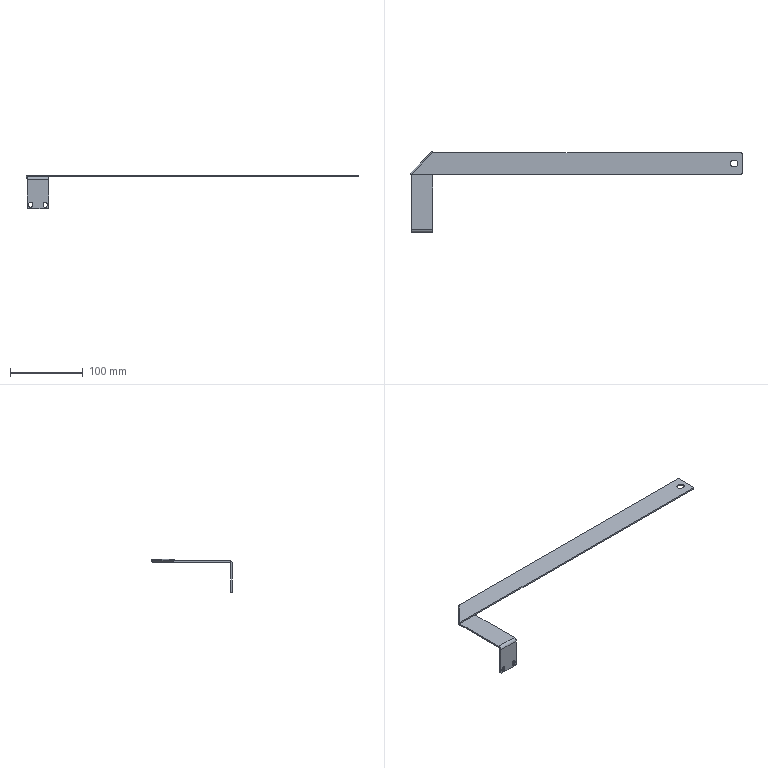Part | NX | features BREP 1 | 1 solid | 37 faces | box 457.646 x 111.304 x 46.082 mm | volume 34595 mm3 | plane 20 | cylinder 17 | commonest cylinder face diameters 5.5 x6 4 x5 9 x3 2 x2 8 x1
STEP:
#1=CARTESIAN_POINT('',(-257.062,-128.404,2032.018));
#2=VERTEX_POINT('',#1);
#3=CARTESIAN_POINT('',(-258.476,-126.99,2034.018));
#4=VERTEX_POINT('',#3);
#5=CARTESIAN_POINT('',(-257.062,-128.404,2034.018));
#6=DIRECTION('',(0.7071,0.7071,0.));
#7=DIRECTION('',(-0.7071,0.7071,0.));
#8=AXIS2_PLACEMENT_3D('',#5,#6,#7);
#9=CIRCLE('',#8,2.);
#10=EDGE_CURVE('',#2,#4,#9,.T.);
#11=ORIENTED_EDGE('',*,*,#10,.T.);
#12=CARTESIAN_POINT('',(-228.476,-96.99,2034.018));
#13=VERTEX_POINT('',#12);
#14=CARTESIAN_POINT('',(-258.476,-126.99,2034.018));
#15=DIRECTION('',(0.7071,0.7071,0.));
#16=VECTOR('',#15,1000.);
#17=LINE('',#14,#16);
#18=EDGE_CURVE('',#4,#13,#17,.T.);
#19=ORIENTED_EDGE('',*,*,#18,.T.);
#20=CARTESIAN_POINT('',(-227.062,-98.404,2032.018));
#21=VERTEX_POINT('',#20);
#22=CARTESIAN_POINT('',(-227.062,-98.404,2034.018));
#23=DIRECTION('',(-0.7071,-0.7071,0.));
#24=DIRECTION('',(-0.7071,0.7071,0.));
#25=AXIS2_PLACEMENT_3D('',#22,#23,#24);
#26=CIRCLE('',#25,2.);
#27=EDGE_CURVE('',#13,#21,#26,.T.);
#28=ORIENTED_EDGE('',*,*,#27,.T.);
#29=CARTESIAN_POINT('',(-257.062,-128.404,2032.018));
#30=DIRECTION('',(-0.7071,-0.7071,0.));
#31=VECTOR('',#30,1000.);
#32=LINE('',#29,#31);
#33=EDGE_CURVE('',#21,#2,#32,.T.);
#34=ORIENTED_EDGE('',*,*,#33,.T.);
#35=EDGE_LOOP('',(#11,#19,#28,#34));
#36=FACE_BOUND('',#35,.T.);
#37=CARTESIAN_POINT('',(-257.062,-128.404,2034.018));
#38=DIRECTION('',(0.7071,0.7071,0.));
#39=DIRECTION('',(0.7071,-0.7071,0.));
#40=AXIS2_PLACEMENT_3D('',#37,#38,#39);
#41=CYLINDRICAL_SURFACE('',#40,2.);
#42=ADVANCED_FACE('',(#36),#41,.T.);
#43=CARTESIAN_POINT('',(193.42,-113.404,2034.018));
#44=VERTEX_POINT('',#43);
#45=CARTESIAN_POINT('',(188.92,-108.904,2034.018));
#46=VERTEX_POINT('',#45);
#47=CARTESIAN_POINT('',(188.92,-113.404,2034.018));
#48=DIRECTION('',(0.,0.,1.));
#49=DIRECTION('',(1.,0.,0.));
#50=AXIS2_PLACEMENT_3D('',#47,#48,#49);
#51=CIRCLE('',#50,4.5);
#52=EDGE_CURVE('',#44,#46,#51,.T.);
#53=ORIENTED_EDGE('',*,*,#52,.F.);
#54=CARTESIAN_POINT('',(193.42,-113.404,2036.018));
#55=VERTEX_POINT('',#54);
#56=CARTESIAN_POINT('',(193.42,-113.404,2035.018));
#57=DIRECTION('',(0.,0.,1.));
#58=VECTOR('',#57,1000.);
#59=LINE('',#56,#58);
#60=EDGE_CURVE('',#44,#55,#59,.T.);
#61=ORIENTED_EDGE('',*,*,#60,.T.);
#62=CARTESIAN_POINT('',(188.92,-108.904,2036.018));
#63=VERTEX_POINT('',#62);
#64=CARTESIAN_POINT('',(188.92,-113.404,2036.018));
#65=DIRECTION('',(0.,0.,1.));
#66=DIRECTION('',(1.,0.,0.));
#67=AXIS2_PLACEMENT_3D('',#64,#65,#66);
#68=CIRCLE('',#67,4.5);
#69=EDGE_CURVE('',#55,#63,#68,.T.);
#70=ORIENTED_EDGE('',*,*,#69,.T.);
#71=CARTESIAN_POINT('',(188.92,-108.904,2035.018));
#72=DIRECTION('',(0.,0.,1.));
#73=VECTOR('',#72,1000.);
#74=LINE('',#71,#73);
#75=EDGE_CURVE('',#46,#63,#74,.T.);
#76=ORIENTED_EDGE('',*,*,#75,.F.);
#77=EDGE_LOOP('',(#53,#61,#70,#76));
#78=FACE_BOUND('',#77,.T.);
#79=CARTESIAN_POINT('',(188.92,-113.404,2035.018));
#80=DIRECTION('',(0.,0.,1.));
#81=DIRECTION('',(-1.,0.,0.));
#82=AXIS2_PLACEMENT_3D('',#79,#80,#81);
#83=CYLINDRICAL_SURFACE('',#82,4.5);
#84=ADVANCED_FACE('',(#78),#83,.F.);
#85=CARTESIAN_POINT('',(-229.312,-206.294,1994.768));
#86=VERTEX_POINT('',#85);
#87=CARTESIAN_POINT('',(-232.062,-206.294,1992.018));
#88=VERTEX_POINT('',#87);
#89=CARTESIAN_POINT('',(-232.062,-206.294,1994.768));
#90=DIRECTION('',(0.,1.,0.));
#91=DIRECTION('',(0.,0.,-1.));
#92=AXIS2_PLACEMENT_3D('',#89,#90,#91);
#93=CIRCLE('',#92,2.75);
#94=EDGE_CURVE('',#86,#88,#93,.T.);
#95=ORIENTED_EDGE('',*,*,#94,.T.);
#96=CARTESIAN_POINT('',(-232.062,-208.294,1992.018));
#97=VERTEX_POINT('',#96);
#98=CARTESIAN_POINT('',(-232.062,-207.294,1992.018));
#99=DIRECTION('',(0.,-1.,0.));
#100=VECTOR('',#99,1000.);
#101=LINE('',#98,#100);
#102=EDGE_CURVE('',#88,#97,#101,.T.);
#103=ORIENTED_EDGE('',*,*,#102,.T.);
#104=CARTESIAN_POINT('',(-229.312,-208.294,1994.768));
#105=VERTEX_POINT('',#104);
#106=CARTESIAN_POINT('',(-232.062,-208.294,1994.768));
#107=DIRECTION('',(0.,1.,0.));
#108=DIRECTION('',(0.,0.,-1.));
#109=AXIS2_PLACEMENT_3D('',#106,#107,#108);
#110=CIRCLE('',#109,2.75);
#111=EDGE_CURVE('',#105,#97,#110,.T.);
#112=ORIENTED_EDGE('',*,*,#111,.F.);
#113=CARTESIAN_POINT('',(-229.312,-207.294,1994.768));
#114=DIRECTION('',(0.,-1.,0.));
#115=VECTOR('',#114,1000.);
#116=LINE('',#113,#115);
#117=EDGE_CURVE('',#86,#105,#116,.T.);
#118=ORIENTED_EDGE('',*,*,#117,.F.);
#119=EDGE_LOOP('',(#95,#103,#112,#118));
#120=FACE_BOUND('',#119,.T.);
#121=CARTESIAN_POINT('',(-232.062,-207.294,1994.768));
#122=DIRECTION('',(0.,-1.,0.));
#123=DIRECTION('',(0.,0.,1.));
#124=AXIS2_PLACEMENT_3D('',#121,#122,#123);
#125=CYLINDRICAL_SURFACE('',#124,2.75);
#126=ADVANCED_FACE('',(#120),#125,.F.);
#127=CARTESIAN_POINT('',(-249.312,-206.294,1994.768));
#128=VERTEX_POINT('',#127);
#129=CARTESIAN_POINT('',(-252.062,-206.294,1992.018));
#130=VERTEX_POINT('',#129);
#131=CARTESIAN_POINT('',(-252.062,-206.294,1994.768));
#132=DIRECTION('',(0.,1.,0.));
#133=DIRECTION('',(0.,0.,-1.));
#134=AXIS2_PLACEMENT_3D('',#131,#132,#133);
#135=CIRCLE('',#134,2.75);
#136=EDGE_CURVE('',#128,#130,#135,.T.);
#137=ORIENTED_EDGE('',*,*,#136,.T.);
#138=CARTESIAN_POINT('',(-252.062,-208.294,1992.018));
#139=VERTEX_POINT('',#138);
#140=CARTESIAN_POINT('',(-252.062,-207.294,1992.018));
#141=DIRECTION('',(0.,-1.,0.));
#142=VECTOR('',#141,1000.);
#143=LINE('',#140,#142);
#144=EDGE_CURVE('',#130,#139,#143,.T.);
#145=ORIENTED_EDGE('',*,*,#144,.T.);
#146=CARTESIAN_POINT('',(-249.312,-208.294,1994.768));
#147=VERTEX_POINT('',#146);
#148=CARTESIAN_POINT('',(-252.062,-208.294,1994.768));
#149=DIRECTION('',(0.,1.,0.));
#150=DIRECTION('',(0.,0.,-1.));
#151=AXIS2_PLACEMENT_3D('',#148,#149,#150);
#152=CIRCLE('',#151,2.75);
#153=EDGE_CURVE('',#147,#139,#152,.T.);
#154=ORIENTED_EDGE('',*,*,#153,.F.);
#155=CARTESIAN_POINT('',(-249.312,-207.294,1994.768));
#156=DIRECTION('',(0.,-1.,0.));
#157=VECTOR('',#156,1000.);
#158=LINE('',#155,#157);
#159=EDGE_CURVE('',#128,#147,#158,.T.);
#160=ORIENTED_EDGE('',*,*,#159,.F.);
#161=EDGE_LOOP('',(#137,#145,#154,#160));
#162=FACE_BOUND('',#161,.T.);
#163=CARTESIAN_POINT('',(-252.062,-207.294,1994.768));
#164=DIRECTION('',(0.,-1.,0.));
#165=DIRECTION('',(0.,0.,1.));
#166=AXIS2_PLACEMENT_3D('',#163,#164,#165);
#167=CYLINDRICAL_SURFACE('',#166,2.75);
#168=ADVANCED_FACE('',(#162),#167,.F.);
#169=CARTESIAN_POINT('',(198.17,-128.404,2036.018));
#170=VERTEX_POINT('',#169);
#171=CARTESIAN_POINT('',(-257.062,-128.404,2036.018));
#172=VERTEX_POINT('',#171);
#173=CARTESIAN_POINT('',(-234.19,-128.404,2036.018));
#174=DIRECTION('',(-1.,0.,0.));
#175=VECTOR('',#174,1000.);
#176=LINE('',#173,#175);
#177=EDGE_CURVE('',#170,#172,#176,.T.);
#178=ORIENTED_EDGE('',*,*,#177,.F.);
#179=CARTESIAN_POINT('',(199.17,-127.404,2036.018));
#180=VERTEX_POINT('',#179);
#181=CARTESIAN_POINT('',(198.17,-127.404,2036.018));
#182=DIRECTION('',(0.,0.,-1.));
#183=DIRECTION('',(1.,0.,0.));
#184=AXIS2_PLACEMENT_3D('',#181,#182,#183);
#185=CIRCLE('',#184,1.);
#186=EDGE_CURVE('',#180,#170,#185,.T.);
#187=ORIENTED_EDGE('',*,*,#186,.F.);
#188=CARTESIAN_POINT('',(199.17,-99.404,2036.018));
#189=VERTEX_POINT('',#188);
#190=CARTESIAN_POINT('',(199.17,-105.532,2036.018));
#191=DIRECTION('',(0.,-1.,0.));
#192=VECTOR('',#191,1000.);
#193=LINE('',#190,#192);
#194=EDGE_CURVE('',#189,#180,#193,.T.);
#195=ORIENTED_EDGE('',*,*,#194,.F.);
#196=CARTESIAN_POINT('',(198.17,-98.404,2036.018));
#197=VERTEX_POINT('',#196);
#198=CARTESIAN_POINT('',(198.17,-99.404,2036.018));
#199=DIRECTION('',(0.,0.,-1.));
#200=DIRECTION('',(1.,0.,0.));
#201=AXIS2_PLACEMENT_3D('',#198,#199,#200);
#202=CIRCLE('',#201,1.);
#203=EDGE_CURVE('',#197,#189,#202,.T.);
#204=ORIENTED_EDGE('',*,*,#203,.F.);
#205=CARTESIAN_POINT('',(-227.062,-98.404,2036.018));
#206=VERTEX_POINT('',#205);
#207=CARTESIAN_POINT('',(-234.19,-98.404,2036.018));
#208=DIRECTION('',(1.,0.,0.));
#209=VECTOR('',#208,1000.);
#210=LINE('',#207,#209);
#211=EDGE_CURVE('',#206,#197,#210,.T.);
#212=ORIENTED_EDGE('',*,*,#211,.F.);
#213=CARTESIAN_POINT('',(-257.062,-128.404,2036.018));
#214=DIRECTION('',(0.7071,0.7071,0.));
#215=VECTOR('',#214,1000.);
#216=LINE('',#213,#215);
#217=EDGE_CURVE('',#172,#206,#216,.T.);
#218=ORIENTED_EDGE('',*,*,#217,.F.);
#219=EDGE_LOOP('',(#178,#187,#195,#204,#212,#218));
#220=FACE_BOUND('',#219,.T.);
#221=CARTESIAN_POINT('',(187.42,-108.904,2036.018));
#222=VERTEX_POINT('',#221);
#223=CARTESIAN_POINT('',(188.17,-108.904,2036.018));
#224=DIRECTION('',(-1.,0.,0.));
#225=VECTOR('',#224,1000.);
#226=LINE('',#223,#225);
#227=EDGE_CURVE('',#63,#222,#226,.T.);
#228=ORIENTED_EDGE('',*,*,#227,.F.);
#229=ORIENTED_EDGE('',*,*,#69,.F.);
#230=CARTESIAN_POINT('',(188.92,-117.904,2036.018));
#231=VERTEX_POINT('',#230);
#232=CARTESIAN_POINT('',(188.92,-113.404,2036.018));
#233=DIRECTION('',(0.,0.,1.));
#234=DIRECTION('',(1.,0.,0.));
#235=AXIS2_PLACEMENT_3D('',#232,#233,#234);
#236=CIRCLE('',#235,4.5);
#237=EDGE_CURVE('',#231,#55,#236,.T.);
#238=ORIENTED_EDGE('',*,*,#237,.F.);
#239=CARTESIAN_POINT('',(187.42,-117.904,2036.018));
#240=VERTEX_POINT('',#239);
#241=CARTESIAN_POINT('',(188.17,-117.904,2036.018));
#242=DIRECTION('',(1.,0.,0.));
#243=VECTOR('',#242,1000.);
#244=LINE('',#241,#243);
#245=EDGE_CURVE('',#240,#231,#244,.T.);
#246=ORIENTED_EDGE('',*,*,#245,.F.);
#247=CARTESIAN_POINT('',(187.42,-113.404,2036.018));
#248=DIRECTION('',(0.,0.,1.));
#249=DIRECTION('',(1.,0.,0.));
#250=AXIS2_PLACEMENT_3D('',#247,#248,#249);
#251=CIRCLE('',#250,4.5);
#252=EDGE_CURVE('',#222,#240,#251,.T.);
#253=ORIENTED_EDGE('',*,*,#252,.F.);
#254=EDGE_LOOP('',(#228,#229,#238,#246,#253));
#255=FACE_BOUND('',#254,.T.);
#256=CARTESIAN_POINT('',(-234.19,-105.532,2036.018));
#257=DIRECTION('',(0.,0.,-1.));
#258=DIRECTION('',(1.,0.,0.));
#259=AXIS2_PLACEMENT_3D('',#256,#257,#258);
#260=PLANE('',#259);
#261=ADVANCED_FACE('',(#220,#255),#260,.F.);
#262=ORIENTED_EDGE('',*,*,#18,.F.);
#263=CARTESIAN_POINT('',(-257.062,-128.404,2034.018));
#264=DIRECTION('',(0.7071,0.7071,0.));
#265=DIRECTION('',(-0.7071,0.7071,0.));
#266=AXIS2_PLACEMENT_3D('',#263,#264,#265);
#267=CIRCLE('',#266,2.);
#268=EDGE_CURVE('',#4,#172,#267,.T.);
#269=ORIENTED_EDGE('',*,*,#268,.T.);
#270=ORIENTED_EDGE('',*,*,#217,.T.);
#271=CARTESIAN_POINT('',(-227.062,-98.404,2034.018));
#272=DIRECTION('',(-0.7071,-0.7071,0.));
#273=DIRECTION('',(-0.7071,0.7071,0.));
#274=AXIS2_PLACEMENT_3D('',#271,#272,#273);
#275=CIRCLE('',#274,2.);
#276=EDGE_CURVE('',#206,#13,#275,.T.);
#277=ORIENTED_EDGE('',*,*,#276,.T.);
#278=EDGE_LOOP('',(#262,#269,#270,#277));
#279=FACE_BOUND('',#278,.T.);
#280=CARTESIAN_POINT('',(-257.062,-128.404,2034.018));
#281=DIRECTION('',(0.7071,0.7071,0.));
#282=DIRECTION('',(0.7071,-0.7071,0.));
#283=AXIS2_PLACEMENT_3D('',#280,#281,#282);
#284=CYLINDRICAL_SURFACE('',#283,2.);
#285=ADVANCED_FACE('',(#279),#284,.T.);
#286=ORIENTED_EDGE('',*,*,#177,.T.);
#287=CARTESIAN_POINT('',(-257.062,-128.404,2034.018));
#288=VERTEX_POINT('',#287);
#289=CARTESIAN_POINT('',(-257.062,-128.404,2035.018));
#290=DIRECTION('',(0.,0.,-1.));
#291=VECTOR('',#290,1000.);
#292=LINE('',#289,#291);
#293=EDGE_CURVE('',#172,#288,#292,.T.);
#294=ORIENTED_EDGE('',*,*,#293,.T.);
#295=CARTESIAN_POINT('',(198.17,-128.404,2034.018));
#296=VERTEX_POINT('',#295);
#297=CARTESIAN_POINT('',(-6.297,-128.404,2034.018));
#298=DIRECTION('',(1.,0.,0.));
#299=VECTOR('',#298,1000.);
#300=LINE('',#297,#299);
#301=EDGE_CURVE('',#288,#296,#300,.T.);
#302=ORIENTED_EDGE('',*,*,#301,.T.);
#303=CARTESIAN_POINT('',(198.17,-128.404,2035.018));
#304=DIRECTION('',(0.,0.,1.));
#305=VECTOR('',#304,1000.);
#306=LINE('',#303,#305);
#307=EDGE_CURVE('',#296,#170,#306,.T.);
#308=ORIENTED_EDGE('',*,*,#307,.T.);
#309=EDGE_LOOP('',(#286,#294,#302,#308));
#310=FACE_BOUND('',#309,.T.);
#311=CARTESIAN_POINT('',(-6.297,-128.404,2035.018));
#312=DIRECTION('',(0.,-1.,0.));
#313=DIRECTION('',(0.,0.,1.));
#314=AXIS2_PLACEMENT_3D('',#311,#312,#313);
#315=PLANE('',#314);
#316=ADVANCED_FACE('',(#310),#315,.T.);
#317=CARTESIAN_POINT('',(199.17,-127.404,2034.018));
#318=VERTEX_POINT('',#317);
#319=CARTESIAN_POINT('',(199.17,-127.404,2035.018));
#320=DIRECTION('',(0.,0.,-1.));
#321=VECTOR('',#320,1000.);
#322=LINE('',#319,#321);
#323=EDGE_CURVE('',#180,#318,#322,.T.);
#324=ORIENTED_EDGE('',*,*,#323,.T.);
#325=CARTESIAN_POINT('',(199.17,-99.404,2034.018));
#326=VERTEX_POINT('',#325);
#327=CARTESIAN_POINT('',(199.17,-113.404,2034.018));
#328=DIRECTION('',(0.,1.,0.));
#329=VECTOR('',#328,1000.);
#330=LINE('',#327,#329);
#331=EDGE_CURVE('',#318,#326,#330,.T.);
#332=ORIENTED_EDGE('',*,*,#331,.T.);
#333=CARTESIAN_POINT('',(199.17,-99.404,2035.018));
#334=DIRECTION('',(0.,0.,1.));
#335=VECTOR('',#334,1000.);
#336=LINE('',#333,#335);
#337=EDGE_CURVE('',#326,#189,#336,.T.);
#338=ORIENTED_EDGE('',*,*,#337,.T.);
#339=ORIENTED_EDGE('',*,*,#194,.T.);
#340=EDGE_LOOP('',(#324,#332,#338,#339));
#341=FACE_BOUND('',#340,.T.);
#342=CARTESIAN_POINT('',(199.17,-113.404,2035.018));
#343=DIRECTION('',(1.,0.,0.));
#344=DIRECTION('',(0.,0.,1.));
#345=AXIS2_PLACEMENT_3D('',#342,#343,#344);
#346=PLANE('',#345);
#347=ADVANCED_FACE('',(#341),#346,.T.);
#348=CARTESIAN_POINT('',(198.17,-98.404,2034.018));
#349=VERTEX_POINT('',#348);
#350=CARTESIAN_POINT('',(-227.062,-98.404,2034.018));
#351=VERTEX_POINT('',#350);
#352=CARTESIAN_POINT('',(8.703,-98.404,2034.018));
#353=DIRECTION('',(-1.,0.,0.));
#354=VECTOR('',#353,1000.);
#355=LINE('',#352,#354);
#356=EDGE_CURVE('',#349,#351,#355,.T.);
#357=ORIENTED_EDGE('',*,*,#356,.T.);
#358=CARTESIAN_POINT('',(-227.062,-98.404,2035.018));
#359=DIRECTION('',(0.,0.,1.));
#360=VECTOR('',#359,1000.);
#361=LINE('',#358,#360);
#362=EDGE_CURVE('',#351,#206,#361,.T.);
#363=ORIENTED_EDGE('',*,*,#362,.T.);
#364=ORIENTED_EDGE('',*,*,#211,.T.);
#365=CARTESIAN_POINT('',(198.17,-98.404,2035.018));
#366=DIRECTION('',(0.,0.,-1.));
#367=VECTOR('',#366,1000.);
#368=LINE('',#365,#367);
#369=EDGE_CURVE('',#197,#349,#368,.T.);
#370=ORIENTED_EDGE('',*,*,#369,.T.);
#371=EDGE_LOOP('',(#357,#363,#364,#370));
#372=FACE_BOUND('',#371,.T.);
#373=CARTESIAN_POINT('',(8.703,-98.404,2035.018));
#374=DIRECTION('',(0.,1.,0.));
#375=DIRECTION('',(0.,0.,-1.));
#376=AXIS2_PLACEMENT_3D('',#373,#374,#375);
#377=PLANE('',#376);
#378=ADVANCED_FACE('',(#372),#377,.T.);
#379=ORIENTED_EDGE('',*,*,#60,.F.);
#380=CARTESIAN_POINT('',(188.92,-117.904,2034.018));
#381=VERTEX_POINT('',#380);
#382=CARTESIAN_POINT('',(188.92,-113.404,2034.018));
#383=DIRECTION('',(0.,0.,1.));
#384=DIRECTION('',(1.,0.,0.));
#385=AXIS2_PLACEMENT_3D('',#382,#383,#384);
#386=CIRCLE('',#385,4.5);
#387=EDGE_CURVE('',#381,#44,#386,.T.);
#388=ORIENTED_EDGE('',*,*,#387,.F.);
#389=CARTESIAN_POINT('',(188.92,-117.904,2035.018));
#390=DIRECTION('',(0.,0.,-1.));
#391=VECTOR('',#390,1000.);
#392=LINE('',#389,#391);
#393=EDGE_CURVE('',#231,#381,#392,.T.);
#394=ORIENTED_EDGE('',*,*,#393,.F.);
#395=ORIENTED_EDGE('',*,*,#237,.T.);
#396=EDGE_LOOP('',(#379,#388,#394,#395));
#397=FACE_BOUND('',#396,.T.);
#398=CARTESIAN_POINT('',(188.92,-113.404,2035.018));
#399=DIRECTION('',(0.,0.,1.));
#400=DIRECTION('',(-1.,0.,0.));
#401=AXIS2_PLACEMENT_3D('',#398,#399,#400);
#402=CYLINDRICAL_SURFACE('',#401,4.5);
#403=ADVANCED_FACE('',(#397),#402,.F.);
#404=CARTESIAN_POINT('',(187.42,-108.904,2034.018));
#405=VERTEX_POINT('',#404);
#406=CARTESIAN_POINT('',(187.42,-108.904,2035.018));
#407=DIRECTION('',(0.,0.,-1.));
#408=VECTOR('',#407,1000.);
#409=LINE('',#406,#408);
#410=EDGE_CURVE('',#222,#405,#409,.T.);
#411=ORIENTED_EDGE('',*,*,#410,.F.);
#412=ORIENTED_EDGE('',*,*,#252,.T.);
#413=CARTESIAN_POINT('',(187.42,-117.904,2034.018));
#414=VERTEX_POINT('',#413);
#415=CARTESIAN_POINT('',(187.42,-117.904,2035.018));
#416=DIRECTION('',(0.,0.,1.));
#417=VECTOR('',#416,1000.);
#418=LINE('',#415,#417);
#419=EDGE_CURVE('',#414,#240,#418,.T.);
#420=ORIENTED_EDGE('',*,*,#419,.F.);
#421=CARTESIAN_POINT('',(187.42,-113.404,2034.018));
#422=DIRECTION('',(0.,0.,1.));
#423=DIRECTION('',(1.,0.,0.));
#424=AXIS2_PLACEMENT_3D('',#421,#422,#423);
#425=CIRCLE('',#424,4.5);
#426=EDGE_CURVE('',#405,#414,#425,.T.);
#427=ORIENTED_EDGE('',*,*,#426,.F.);
#428=EDGE_LOOP('',(#411,#412,#420,#427));
#429=FACE_BOUND('',#428,.T.);
#430=CARTESIAN_POINT('',(187.42,-113.404,2035.018));
#431=DIRECTION('',(0.,0.,1.));
#432=DIRECTION('',(-1.,0.,0.));
#433=AXIS2_PLACEMENT_3D('',#430,#431,#432);
#434=CYLINDRICAL_SURFACE('',#433,4.5);
#435=ADVANCED_FACE('',(#429),#434,.F.);
#436=CARTESIAN_POINT('',(-227.062,-98.404,2034.018));
#437=DIRECTION('',(0.,0.,-1.));
#438=VECTOR('',#437,1000.);
#439=LINE('',#436,#438);
#440=EDGE_CURVE('',#351,#21,#439,.T.);
#441=ORIENTED_EDGE('',*,*,#440,.T.);
#442=ORIENTED_EDGE('',*,*,#27,.F.);
#443=ORIENTED_EDGE('',*,*,#276,.F.);
#444=ORIENTED_EDGE('',*,*,#362,.F.);
#445=EDGE_LOOP('',(#441,#442,#443,#444));
#446=FACE_BOUND('',#445,.T.);
#447=CARTESIAN_POINT('',(-227.769,-97.697,2034.018));
#448=DIRECTION('',(0.7071,0.7071,0.));
#449=DIRECTION('',(0.7071,-0.7071,0.));
#450=AXIS2_PLACEMENT_3D('',#447,#448,#449);
#451=PLANE('',#450);
#452=ADVANCED_FACE('',(#446),#451,.T.);
#453=ORIENTED_EDGE('',*,*,#10,.F.);
#454=CARTESIAN_POINT('',(-257.062,-128.404,2034.018));
#455=DIRECTION('',(0.,0.,1.));
#456=VECTOR('',#455,1000.);
#457=LINE('',#454,#456);
#458=EDGE_CURVE('',#2,#288,#457,.T.);
#459=ORIENTED_EDGE('',*,*,#458,.T.);
#460=ORIENTED_EDGE('',*,*,#293,.F.);
#461=ORIENTED_EDGE('',*,*,#268,.F.);
#462=EDGE_LOOP('',(#453,#459,#460,#461));
#463=FACE_BOUND('',#462,.T.);
#464=CARTESIAN_POINT('',(-257.769,-127.697,2034.018));
#465=DIRECTION('',(-0.7071,-0.7071,0.));
#466=DIRECTION('',(-0.7071,0.7071,0.));
#467=AXIS2_PLACEMENT_3D('',#464,#465,#466);
#468=PLANE('',#467);
#469=ADVANCED_FACE('',(#463),#468,.T.);
#470=CARTESIAN_POINT('',(198.17,-127.404,2034.018));
#471=DIRECTION('',(0.,0.,1.));
#472=DIRECTION('',(1.,0.,0.));
#473=AXIS2_PLACEMENT_3D('',#470,#471,#472);
#474=CIRCLE('',#473,1.);
#475=EDGE_CURVE('',#296,#318,#474,.T.);
#476=ORIENTED_EDGE('',*,*,#475,.T.);
#477=ORIENTED_EDGE('',*,*,#323,.F.);
#478=ORIENTED_EDGE('',*,*,#186,.T.);
#479=ORIENTED_EDGE('',*,*,#307,.F.);
#480=EDGE_LOOP('',(#476,#477,#478,#479));
#481=FACE_BOUND('',#480,.T.);
#482=CARTESIAN_POINT('',(198.17,-127.404,2035.018));
#483=DIRECTION('',(0.,0.,1.));
#484=DIRECTION('',(-1.,0.,0.));
#485=AXIS2_PLACEMENT_3D('',#482,#483,#484);
#486=CYLINDRICAL_SURFACE('',#485,1.);
#487=ADVANCED_FACE('',(#481),#486,.T.);
#488=ORIENTED_EDGE('',*,*,#356,.F.);
#489=CARTESIAN_POINT('',(198.17,-99.404,2034.018));
#490=DIRECTION('',(0.,0.,1.));
#491=DIRECTION('',(1.,0.,0.));
#492=AXIS2_PLACEMENT_3D('',#489,#490,#491);
#493=CIRCLE('',#492,1.);
#494=EDGE_CURVE('',#326,#349,#493,.T.);
#495=ORIENTED_EDGE('',*,*,#494,.F.);
#496=ORIENTED_EDGE('',*,*,#331,.F.);
#497=ORIENTED_EDGE('',*,*,#475,.F.);
#498=ORIENTED_EDGE('',*,*,#301,.F.);
#499=CARTESIAN_POINT('',(-227.062,-98.404,2034.018));
#500=DIRECTION('',(-0.7071,-0.7071,0.));
#501=VECTOR('',#500,1000.);
#502=LINE('',#499,#501);
#503=EDGE_CURVE('',#351,#288,#502,.T.);
#504=ORIENTED_EDGE('',*,*,#503,.F.);
#505=EDGE_LOOP('',(#488,#495,#496,#497,#498,#504));
#506=FACE_BOUND('',#505,.T.);
#507=ORIENTED_EDGE('',*,*,#426,.T.);
#508=CARTESIAN_POINT('',(-227.062,-117.904,2034.018));
#509=DIRECTION('',(-1.,0.,0.));
#510=VECTOR('',#509,1000.);
#511=LINE('',#508,#510);
#512=EDGE_CURVE('',#381,#414,#511,.T.);
#513=ORIENTED_EDGE('',*,*,#512,.F.);
#514=ORIENTED_EDGE('',*,*,#387,.T.);
#515=ORIENTED_EDGE('',*,*,#52,.T.);
#516=CARTESIAN_POINT('',(-227.062,-108.904,2034.018));
#517=DIRECTION('',(1.,0.,0.));
#518=VECTOR('',#517,1000.);
#519=LINE('',#516,#518);
#520=EDGE_CURVE('',#405,#46,#519,.T.);
#521=ORIENTED_EDGE('',*,*,#520,.F.);
#522=EDGE_LOOP('',(#507,#513,#514,#515,#521));
#523=FACE_BOUND('',#522,.T.);
#524=CARTESIAN_POINT('',(-227.062,-208.294,2034.018));
#525=DIRECTION('',(0.,0.,1.));
#526=DIRECTION('',(-1.,0.,0.));
#527=AXIS2_PLACEMENT_3D('',#524,#525,#526);
#528=PLANE('',#527);
#529=ADVANCED_FACE('',(#506,#523),#528,.F.);
#530=ORIENTED_EDGE('',*,*,#494,.T.);
#531=ORIENTED_EDGE('',*,*,#369,.F.);
#532=ORIENTED_EDGE('',*,*,#203,.T.);
#533=ORIENTED_EDGE('',*,*,#337,.F.);
#534=EDGE_LOOP('',(#530,#531,#532,#533));
#535=FACE_BOUND('',#534,.T.);
#536=CARTESIAN_POINT('',(198.17,-99.404,2035.018));
#537=DIRECTION('',(0.,0.,1.));
#538=DIRECTION('',(-1.,0.,0.));
#539=AXIS2_PLACEMENT_3D('',#536,#537,#538);
#540=CYLINDRICAL_SURFACE('',#539,1.);
#541=ADVANCED_FACE('',(#535),#540,.T.);
#542=ORIENTED_EDGE('',*,*,#520,.T.);
#543=ORIENTED_EDGE('',*,*,#75,.T.);
#544=ORIENTED_EDGE('',*,*,#227,.T.);
#545=ORIENTED_EDGE('',*,*,#410,.T.);
#546=EDGE_LOOP('',(#542,#543,#544,#545));
#547=FACE_BOUND('',#546,.T.);
#548=CARTESIAN_POINT('',(188.17,-108.904,2035.018));
#549=DIRECTION('',(0.,-1.,0.));
#550=DIRECTION('',(-1.,0.,0.));
#551=AXIS2_PLACEMENT_3D('',#548,#549,#550);
#552=PLANE('',#551);
#553=ADVANCED_FACE('',(#547),#552,.T.);
#554=ORIENTED_EDGE('',*,*,#512,.T.);
#555=ORIENTED_EDGE('',*,*,#419,.T.);
#556=ORIENTED_EDGE('',*,*,#245,.T.);
#557=ORIENTED_EDGE('',*,*,#393,.T.);
#558=EDGE_LOOP('',(#554,#555,#556,#557));
#559=FACE_BOUND('',#558,.T.);
#560=CARTESIAN_POINT('',(188.17,-117.904,2035.018));
#561=DIRECTION('',(0.,1.,0.));
#562=DIRECTION('',(0.,0.,-1.));
#563=AXIS2_PLACEMENT_3D('',#560,#561,#562);
#564=PLANE('',#563);
#565=ADVANCED_FACE('',(#559),#564,.T.);
#566=ORIENTED_EDGE('',*,*,#440,.F.);
#567=CARTESIAN_POINT('',(-227.062,-204.294,2034.018));
#568=VERTEX_POINT('',#567);
#569=CARTESIAN_POINT('',(-227.062,-207.294,2034.018));
#570=DIRECTION('',(0.,1.,0.));
#571=VECTOR('',#570,1000.);
#572=LINE('',#569,#571);
#573=EDGE_CURVE('',#568,#351,#572,.T.);
#574=ORIENTED_EDGE('',*,*,#573,.F.);
#575=CARTESIAN_POINT('',(-227.062,-208.294,2030.018));
#576=VERTEX_POINT('',#575);
#577=CARTESIAN_POINT('',(-227.062,-204.294,2030.018));
#578=DIRECTION('',(-1.,0.,0.));
#579=DIRECTION('',(0.,0.,-1.));
#580=AXIS2_PLACEMENT_3D('',#577,#578,#579);
#581=CIRCLE('',#580,4.);
#582=EDGE_CURVE('',#576,#568,#581,.T.);
#583=ORIENTED_EDGE('',*,*,#582,.F.);
#584=CARTESIAN_POINT('',(-227.062,-208.294,1991.936));
#585=VERTEX_POINT('',#584);
#586=CARTESIAN_POINT('',(-227.062,-208.294,2009.468));
#587=DIRECTION('',(0.,0.,1.));
#588=VECTOR('',#587,1000.);
#589=LINE('',#586,#588);
#590=EDGE_CURVE('',#585,#576,#589,.T.);
#591=ORIENTED_EDGE('',*,*,#590,.F.);
#592=CARTESIAN_POINT('',(-227.062,-206.294,1991.936));
#593=VERTEX_POINT('',#592);
#594=CARTESIAN_POINT('',(-227.062,-207.294,1991.936));
#595=DIRECTION('',(0.,-1.,0.));
#596=VECTOR('',#595,1000.);
#597=LINE('',#594,#596);
#598=EDGE_CURVE('',#593,#585,#597,.T.);
#599=ORIENTED_EDGE('',*,*,#598,.F.);
#600=CARTESIAN_POINT('',(-227.062,-206.294,2030.018));
#601=VERTEX_POINT('',#600);
#602=CARTESIAN_POINT('',(-227.062,-206.294,2009.468));
#603=DIRECTION('',(0.,0.,-1.));
#604=VECTOR('',#603,1000.);
#605=LINE('',#602,#604);
#606=EDGE_CURVE('',#601,#593,#605,.T.);
#607=ORIENTED_EDGE('',*,*,#606,.F.);
#608=CARTESIAN_POINT('',(-227.062,-204.294,2032.018));
#609=VERTEX_POINT('',#608);
#610=CARTESIAN_POINT('',(-227.062,-204.294,2030.018));
#611=DIRECTION('',(1.,0.,0.));
#612=DIRECTION('',(0.,0.,-1.));
#613=AXIS2_PLACEMENT_3D('',#610,#611,#612);
#614=CIRCLE('',#613,2.);
#615=EDGE_CURVE('',#609,#601,#614,.T.);
#616=ORIENTED_EDGE('',*,*,#615,.F.);
#617=CARTESIAN_POINT('',(-227.062,-207.294,2032.018));
#618=DIRECTION('',(0.,-1.,0.));
#619=VECTOR('',#618,1000.);
#620=LINE('',#617,#619);
#621=EDGE_CURVE('',#21,#609,#620,.T.);
#622=ORIENTED_EDGE('',*,*,#621,.F.);
#623=EDGE_LOOP('',(#566,#574,#583,#591,#599,#607,#616,#622));
#624=FACE_BOUND('',#623,.T.);
#625=CARTESIAN_POINT('',(-227.062,-207.294,2009.468));
#626=DIRECTION('',(-1.,0.,0.));
#627=DIRECTION('',(0.,0.,-1.));
#628=AXIS2_PLACEMENT_3D('',#625,#626,#627);
#629=PLANE('',#628);
#630=ADVANCED_FACE('',(#624),#629,.F.);
#631=ORIENTED_EDGE('',*,*,#458,.F.);
#632=CARTESIAN_POINT('',(-257.062,-204.294,2032.018));
#633=VERTEX_POINT('',#632);
#634=CARTESIAN_POINT('',(-257.062,-207.294,2032.018));
#635=DIRECTION('',(0.,1.,0.));
#636=VECTOR('',#635,1000.);
#637=LINE('',#634,#636);
#638=EDGE_CURVE('',#633,#2,#637,.T.);
#639=ORIENTED_EDGE('',*,*,#638,.F.);
#640=CARTESIAN_POINT('',(-257.062,-206.294,2030.018));
#641=VERTEX_POINT('',#640);
#642=CARTESIAN_POINT('',(-257.062,-204.294,2030.018));
#643=DIRECTION('',(-1.,0.,0.));
#644=DIRECTION('',(0.,0.,-1.));
#645=AXIS2_PLACEMENT_3D('',#642,#643,#644);
#646=CIRCLE('',#645,2.);
#647=EDGE_CURVE('',#641,#633,#646,.T.);
#648=ORIENTED_EDGE('',*,*,#647,.F.);
#649=CARTESIAN_POINT('',(-257.062,-206.294,1991.936));
#650=VERTEX_POINT('',#649);
#651=CARTESIAN_POINT('',(-257.062,-206.294,2009.468));
#652=DIRECTION('',(0.,0.,1.));
#653=VECTOR('',#652,1000.);
#654=LINE('',#651,#653);
#655=EDGE_CURVE('',#650,#641,#654,.T.);
#656=ORIENTED_EDGE('',*,*,#655,.F.);
#657=CARTESIAN_POINT('',(-257.062,-208.294,1991.936));
#658=VERTEX_POINT('',#657);
#659=CARTESIAN_POINT('',(-257.062,-207.294,1991.936));
#660=DIRECTION('',(0.,1.,0.));
#661=VECTOR('',#660,1000.);
#662=LINE('',#659,#661);
#663=EDGE_CURVE('',#658,#650,#662,.T.);
#664=ORIENTED_EDGE('',*,*,#663,.F.);
#665=CARTESIAN_POINT('',(-257.062,-208.294,2030.018));
#666=VERTEX_POINT('',#665);
#667=CARTESIAN_POINT('',(-257.062,-208.294,2009.468));
#668=DIRECTION('',(0.,0.,-1.));
#669=VECTOR('',#668,1000.);
#670=LINE('',#667,#669);
#671=EDGE_CURVE('',#666,#658,#670,.T.);
#672=ORIENTED_EDGE('',*,*,#671,.F.);
#673=CARTESIAN_POINT('',(-257.062,-204.294,2034.018));
#674=VERTEX_POINT('',#673);
#675=CARTESIAN_POINT('',(-257.062,-204.294,2030.018));
#676=DIRECTION('',(1.,0.,0.));
#677=DIRECTION('',(0.,0.,-1.));
#678=AXIS2_PLACEMENT_3D('',#675,#676,#677);
#679=CIRCLE('',#678,4.);
#680=EDGE_CURVE('',#674,#666,#679,.T.);
#681=ORIENTED_EDGE('',*,*,#680,.F.);
#682=CARTESIAN_POINT('',(-257.062,-207.294,2034.018));
#683=DIRECTION('',(0.,-1.,0.));
#684=VECTOR('',#683,1000.);
#685=LINE('',#682,#684);
#686=EDGE_CURVE('',#288,#674,#685,.T.);
#687=ORIENTED_EDGE('',*,*,#686,.F.);
#688=EDGE_LOOP('',(#631,#639,#648,#656,#664,#672,#681,#687));
#689=FACE_BOUND('',#688,.T.);
#690=CARTESIAN_POINT('',(-257.062,-207.294,2009.468));
#691=DIRECTION('',(1.,0.,0.));
#692=DIRECTION('',(0.,0.,1.));
#693=AXIS2_PLACEMENT_3D('',#690,#691,#692);
#694=PLANE('',#693);
#695=ADVANCED_FACE('',(#689),#694,.F.);
#696=ORIENTED_EDGE('',*,*,#33,.F.);
#697=ORIENTED_EDGE('',*,*,#621,.T.);
#698=CARTESIAN_POINT('',(-227.062,-204.294,2032.018));
#699=DIRECTION('',(1.,0.,0.));
#700=VECTOR('',#699,1000.);
#701=LINE('',#698,#700);
#702=EDGE_CURVE('',#633,#609,#701,.T.);
#703=ORIENTED_EDGE('',*,*,#702,.F.);
#704=ORIENTED_EDGE('',*,*,#638,.T.);
#705=EDGE_LOOP('',(#696,#697,#703,#704));
#706=FACE_BOUND('',#705,.T.);
#707=CARTESIAN_POINT('',(-227.062,-208.294,2032.018));
#708=DIRECTION('',(0.,0.,1.));
#709=DIRECTION('',(-1.,0.,0.));
#710=AXIS2_PLACEMENT_3D('',#707,#708,#709);
#711=PLANE('',#710);
#712=ADVANCED_FACE('',(#706),#711,.F.);
#713=CARTESIAN_POINT('',(-227.062,-204.294,2034.018));
#714=DIRECTION('',(1.,0.,0.));
#715=VECTOR('',#714,1000.);
#716=LINE('',#713,#715);
#717=EDGE_CURVE('',#674,#568,#716,.T.);
#718=ORIENTED_EDGE('',*,*,#717,.T.);
#719=ORIENTED_EDGE('',*,*,#573,.T.);
#720=ORIENTED_EDGE('',*,*,#503,.T.);
#721=ORIENTED_EDGE('',*,*,#686,.T.);
#722=EDGE_LOOP('',(#718,#719,#720,#721));
#723=FACE_BOUND('',#722,.T.);
#724=CARTESIAN_POINT('',(-227.062,-208.294,2034.018));
#725=DIRECTION('',(0.,0.,1.));
#726=DIRECTION('',(-1.,0.,0.));
#727=AXIS2_PLACEMENT_3D('',#724,#725,#726);
#728=PLANE('',#727);
#729=ADVANCED_FACE('',(#723),#728,.T.);
#730=CARTESIAN_POINT('',(-257.062,-208.294,2030.018));
#731=DIRECTION('',(1.,0.,0.));
#732=VECTOR('',#731,1000.);
#733=LINE('',#730,#732);
#734=EDGE_CURVE('',#666,#576,#733,.T.);
#735=ORIENTED_EDGE('',*,*,#734,.T.);
#736=ORIENTED_EDGE('',*,*,#582,.T.);
#737=ORIENTED_EDGE('',*,*,#717,.F.);
#738=ORIENTED_EDGE('',*,*,#680,.T.);
#739=EDGE_LOOP('',(#735,#736,#737,#738));
#740=FACE_BOUND('',#739,.T.);
#741=CARTESIAN_POINT('',(-257.062,-204.294,2030.018));
#742=DIRECTION('',(1.,0.,0.));
#743=DIRECTION('',(0.,0.,1.));
#744=AXIS2_PLACEMENT_3D('',#741,#742,#743);
#745=CYLINDRICAL_SURFACE('',#744,4.);
#746=ADVANCED_FACE('',(#740),#745,.T.);
#747=ORIENTED_EDGE('',*,*,#671,.T.);
#748=CARTESIAN_POINT('',(-255.062,-208.294,1989.936));
#749=VERTEX_POINT('',#748);
#750=CARTESIAN_POINT('',(-255.062,-208.294,1991.936));
#751=DIRECTION('',(0.,-1.,0.));
#752=DIRECTION('',(0.,0.,1.));
#753=AXIS2_PLACEMENT_3D('',#750,#751,#752);
#754=CIRCLE('',#753,2.);
#755=EDGE_CURVE('',#658,#749,#754,.T.);
#756=ORIENTED_EDGE('',*,*,#755,.T.);
#757=CARTESIAN_POINT('',(-229.062,-208.294,1989.936));
#758=VERTEX_POINT('',#757);
#759=CARTESIAN_POINT('',(1.55,-208.294,1989.936));
#760=DIRECTION('',(1.,0.,0.));
#761=VECTOR('',#760,1000.);
#762=LINE('',#759,#761);
#763=EDGE_CURVE('',#749,#758,#762,.T.);
#764=ORIENTED_EDGE('',*,*,#763,.T.);
#765=CARTESIAN_POINT('',(-229.062,-208.294,1991.936));
#766=DIRECTION('',(0.,-1.,0.));
#767=DIRECTION('',(0.,0.,1.));
#768=AXIS2_PLACEMENT_3D('',#765,#766,#767);
#769=CIRCLE('',#768,2.);
#770=EDGE_CURVE('',#758,#585,#769,.T.);
#771=ORIENTED_EDGE('',*,*,#770,.T.);
#772=ORIENTED_EDGE('',*,*,#590,.T.);
#773=ORIENTED_EDGE('',*,*,#734,.F.);
#774=EDGE_LOOP('',(#747,#756,#764,#771,#772,#773));
#775=FACE_BOUND('',#774,.T.);
#776=ORIENTED_EDGE('',*,*,#111,.T.);
#777=CARTESIAN_POINT('',(-234.812,-208.294,1994.768));
#778=VERTEX_POINT('',#777);
#779=CARTESIAN_POINT('',(-232.062,-208.294,1994.768));
#780=DIRECTION('',(0.,1.,0.));
#781=DIRECTION('',(0.,0.,-1.));
#782=AXIS2_PLACEMENT_3D('',#779,#780,#781);
#783=CIRCLE('',#782,2.75);
#784=EDGE_CURVE('',#97,#778,#783,.T.);
#785=ORIENTED_EDGE('',*,*,#784,.T.);
#786=CARTESIAN_POINT('',(-234.812,-208.294,1996.268));
#787=VERTEX_POINT('',#786);
#788=CARTESIAN_POINT('',(-234.812,-208.294,1995.518));
#789=DIRECTION('',(0.,0.,1.));
#790=VECTOR('',#789,1000.);
#791=LINE('',#788,#790);
#792=EDGE_CURVE('',#778,#787,#791,.T.);
#793=ORIENTED_EDGE('',*,*,#792,.T.);
#794=CARTESIAN_POINT('',(-229.312,-208.294,1996.268));
#795=VERTEX_POINT('',#794);
#796=CARTESIAN_POINT('',(-232.062,-208.294,1996.268));
#797=DIRECTION('',(0.,1.,0.));
#798=DIRECTION('',(0.,0.,-1.));
#799=AXIS2_PLACEMENT_3D('',#796,#797,#798);
#800=CIRCLE('',#799,2.75);
#801=EDGE_CURVE('',#787,#795,#800,.T.);
#802=ORIENTED_EDGE('',*,*,#801,.T.);
#803=CARTESIAN_POINT('',(-229.312,-208.294,1995.518));
#804=DIRECTION('',(0.,0.,-1.));
#805=VECTOR('',#804,1000.);
#806=LINE('',#803,#805);
#807=EDGE_CURVE('',#795,#105,#806,.T.);
#808=ORIENTED_EDGE('',*,*,#807,.T.);
#809=EDGE_LOOP('',(#776,#785,#793,#802,#808));
#810=FACE_BOUND('',#809,.T.);
#811=CARTESIAN_POINT('',(-254.812,-208.294,1994.768));
#812=VERTEX_POINT('',#811);
#813=CARTESIAN_POINT('',(-254.812,-208.294,1996.268));
#814=VERTEX_POINT('',#813);
#815=CARTESIAN_POINT('',(-254.812,-208.294,1995.518));
#816=DIRECTION('',(0.,0.,1.));
#817=VECTOR('',#816,1000.);
#818=LINE('',#815,#817);
#819=EDGE_CURVE('',#812,#814,#818,.T.);
#820=ORIENTED_EDGE('',*,*,#819,.T.);
#821=CARTESIAN_POINT('',(-249.312,-208.294,1996.268));
#822=VERTEX_POINT('',#821);
#823=CARTESIAN_POINT('',(-252.062,-208.294,1996.268));
#824=DIRECTION('',(0.,1.,0.));
#825=DIRECTION('',(0.,0.,-1.));
#826=AXIS2_PLACEMENT_3D('',#823,#824,#825);
#827=CIRCLE('',#826,2.75);
#828=EDGE_CURVE('',#814,#822,#827,.T.);
#829=ORIENTED_EDGE('',*,*,#828,.T.);
#830=CARTESIAN_POINT('',(-249.312,-208.294,1995.518));
#831=DIRECTION('',(0.,0.,-1.));
#832=VECTOR('',#831,1000.);
#833=LINE('',#830,#832);
#834=EDGE_CURVE('',#822,#147,#833,.T.);
#835=ORIENTED_EDGE('',*,*,#834,.T.);
#836=ORIENTED_EDGE('',*,*,#153,.T.);
#837=CARTESIAN_POINT('',(-252.062,-208.294,1994.768));
#838=DIRECTION('',(0.,1.,0.));
#839=DIRECTION('',(0.,0.,-1.));
#840=AXIS2_PLACEMENT_3D('',#837,#838,#839);
#841=CIRCLE('',#840,2.75);
#842=EDGE_CURVE('',#139,#812,#841,.T.);
#843=ORIENTED_EDGE('',*,*,#842,.T.);
#844=EDGE_LOOP('',(#820,#829,#835,#836,#843));
#845=FACE_BOUND('',#844,.T.);
#846=CARTESIAN_POINT('',(1.55,-208.294,73.4));
#847=DIRECTION('',(0.,-1.,0.));
#848=DIRECTION('',(0.,0.,1.));
#849=AXIS2_PLACEMENT_3D('',#846,#847,#848);
#850=PLANE('',#849);
#851=ADVANCED_FACE('',(#775,#810,#845),#850,.T.);
#852=ORIENTED_EDGE('',*,*,#770,.F.);
#853=CARTESIAN_POINT('',(-229.062,-206.294,1989.936));
#854=VERTEX_POINT('',#853);
#855=CARTESIAN_POINT('',(-229.062,-207.294,1989.936));
#856=DIRECTION('',(0.,1.,0.));
#857=VECTOR('',#856,1000.);
#858=LINE('',#855,#857);
#859=EDGE_CURVE('',#758,#854,#858,.T.);
#860=ORIENTED_EDGE('',*,*,#859,.T.);
#861=CARTESIAN_POINT('',(-229.062,-206.294,1991.936));
#862=DIRECTION('',(0.,-1.,0.));
#863=DIRECTION('',(0.,0.,1.));
#864=AXIS2_PLACEMENT_3D('',#861,#862,#863);
#865=CIRCLE('',#864,2.);
#866=EDGE_CURVE('',#854,#593,#865,.T.);
#867=ORIENTED_EDGE('',*,*,#866,.T.);
#868=ORIENTED_EDGE('',*,*,#598,.T.);
#869=EDGE_LOOP('',(#852,#860,#867,#868));
#870=FACE_BOUND('',#869,.T.);
#871=CARTESIAN_POINT('',(-229.062,-207.294,1991.936));
#872=DIRECTION('',(0.,1.,0.));
#873=DIRECTION('',(0.,0.,-1.));
#874=AXIS2_PLACEMENT_3D('',#871,#872,#873);
#875=CYLINDRICAL_SURFACE('',#874,2.);
#876=ADVANCED_FACE('',(#870),#875,.T.);
#877=CARTESIAN_POINT('',(-255.062,-206.294,1989.936));
#878=VERTEX_POINT('',#877);
#879=CARTESIAN_POINT('',(1.55,-206.294,1989.936));
#880=DIRECTION('',(1.,0.,0.));
#881=VECTOR('',#880,1000.);
#882=LINE('',#879,#881);
#883=EDGE_CURVE('',#878,#854,#882,.T.);
#884=ORIENTED_EDGE('',*,*,#883,.F.);
#885=CARTESIAN_POINT('',(-255.062,-206.294,1991.936));
#886=DIRECTION('',(0.,-1.,0.));
#887=DIRECTION('',(0.,0.,1.));
#888=AXIS2_PLACEMENT_3D('',#885,#886,#887);
#889=CIRCLE('',#888,2.);
#890=EDGE_CURVE('',#650,#878,#889,.T.);
#891=ORIENTED_EDGE('',*,*,#890,.F.);
#892=ORIENTED_EDGE('',*,*,#655,.T.);
#893=CARTESIAN_POINT('',(1.55,-206.294,2030.018));
#894=DIRECTION('',(-1.,0.,0.));
#895=VECTOR('',#894,1000.);
#896=LINE('',#893,#895);
#897=EDGE_CURVE('',#601,#641,#896,.T.);
#898=ORIENTED_EDGE('',*,*,#897,.F.);
#899=ORIENTED_EDGE('',*,*,#606,.T.);
#900=ORIENTED_EDGE('',*,*,#866,.F.);
#901=EDGE_LOOP('',(#884,#891,#892,#898,#899,#900));
#902=FACE_BOUND('',#901,.T.);
#903=CARTESIAN_POINT('',(-249.312,-206.294,1996.268));
#904=VERTEX_POINT('',#903);
#905=CARTESIAN_POINT('',(-249.312,-206.294,1995.518));
#906=DIRECTION('',(0.,0.,1.));
#907=VECTOR('',#906,1000.);
#908=LINE('',#905,#907);
#909=EDGE_CURVE('',#128,#904,#908,.T.);
#910=ORIENTED_EDGE('',*,*,#909,.T.);
#911=CARTESIAN_POINT('',(-254.812,-206.294,1996.268));
#912=VERTEX_POINT('',#911);
#913=CARTESIAN_POINT('',(-252.062,-206.294,1996.268));
#914=DIRECTION('',(0.,1.,0.));
#915=DIRECTION('',(0.,0.,-1.));
#916=AXIS2_PLACEMENT_3D('',#913,#914,#915);
#917=CIRCLE('',#916,2.75);
#918=EDGE_CURVE('',#912,#904,#917,.T.);
#919=ORIENTED_EDGE('',*,*,#918,.F.);
#920=CARTESIAN_POINT('',(-254.812,-206.294,1994.768));
#921=VERTEX_POINT('',#920);
#922=CARTESIAN_POINT('',(-254.812,-206.294,1995.518));
#923=DIRECTION('',(0.,0.,-1.));
#924=VECTOR('',#923,1000.);
#925=LINE('',#922,#924);
#926=EDGE_CURVE('',#912,#921,#925,.T.);
#927=ORIENTED_EDGE('',*,*,#926,.T.);
#928=CARTESIAN_POINT('',(-252.062,-206.294,1994.768));
#929=DIRECTION('',(0.,1.,0.));
#930=DIRECTION('',(0.,0.,-1.));
#931=AXIS2_PLACEMENT_3D('',#928,#929,#930);
#932=CIRCLE('',#931,2.75);
#933=EDGE_CURVE('',#130,#921,#932,.T.);
#934=ORIENTED_EDGE('',*,*,#933,.F.);
#935=ORIENTED_EDGE('',*,*,#136,.F.);
#936=EDGE_LOOP('',(#910,#919,#927,#934,#935));
#937=FACE_BOUND('',#936,.T.);
#938=CARTESIAN_POINT('',(-229.312,-206.294,1996.268));
#939=VERTEX_POINT('',#938);
#940=CARTESIAN_POINT('',(-229.312,-206.294,1995.518));
#941=DIRECTION('',(0.,0.,1.));
#942=VECTOR('',#941,1000.);
#943=LINE('',#940,#942);
#944=EDGE_CURVE('',#86,#939,#943,.T.);
#945=ORIENTED_EDGE('',*,*,#944,.T.);
#946=CARTESIAN_POINT('',(-234.812,-206.294,1996.268));
#947=VERTEX_POINT('',#946);
#948=CARTESIAN_POINT('',(-232.062,-206.294,1996.268));
#949=DIRECTION('',(0.,1.,0.));
#950=DIRECTION('',(0.,0.,-1.));
#951=AXIS2_PLACEMENT_3D('',#948,#949,#950);
#952=CIRCLE('',#951,2.75);
#953=EDGE_CURVE('',#947,#939,#952,.T.);
#954=ORIENTED_EDGE('',*,*,#953,.F.);
#955=CARTESIAN_POINT('',(-234.812,-206.294,1994.768));
#956=VERTEX_POINT('',#955);
#957=CARTESIAN_POINT('',(-234.812,-206.294,1995.518));
#958=DIRECTION('',(0.,0.,-1.));
#959=VECTOR('',#958,1000.);
#960=LINE('',#957,#959);
#961=EDGE_CURVE('',#947,#956,#960,.T.);
#962=ORIENTED_EDGE('',*,*,#961,.T.);
#963=CARTESIAN_POINT('',(-232.062,-206.294,1994.768));
#964=DIRECTION('',(0.,1.,0.));
#965=DIRECTION('',(0.,0.,-1.));
#966=AXIS2_PLACEMENT_3D('',#963,#964,#965);
#967=CIRCLE('',#966,2.75);
#968=EDGE_CURVE('',#88,#956,#967,.T.);
#969=ORIENTED_EDGE('',*,*,#968,.F.);
#970=ORIENTED_EDGE('',*,*,#94,.F.);
#971=EDGE_LOOP('',(#945,#954,#962,#969,#970));
#972=FACE_BOUND('',#971,.T.);
#973=CARTESIAN_POINT('',(1.55,-206.294,73.4));
#974=DIRECTION('',(0.,-1.,0.));
#975=DIRECTION('',(0.,0.,1.));
#976=AXIS2_PLACEMENT_3D('',#973,#974,#975);
#977=PLANE('',#976);
#978=ADVANCED_FACE('',(#902,#937,#972),#977,.F.);
#979=ORIENTED_EDGE('',*,*,#702,.T.);
#980=ORIENTED_EDGE('',*,*,#615,.T.);
#981=ORIENTED_EDGE('',*,*,#897,.T.);
#982=ORIENTED_EDGE('',*,*,#647,.T.);
#983=EDGE_LOOP('',(#979,#980,#981,#982));
#984=FACE_BOUND('',#983,.T.);
#985=CARTESIAN_POINT('',(-257.062,-204.294,2030.018));
#986=DIRECTION('',(1.,0.,0.));
#987=DIRECTION('',(0.,0.,1.));
#988=AXIS2_PLACEMENT_3D('',#985,#986,#987);
#989=CYLINDRICAL_SURFACE('',#988,2.);
#990=ADVANCED_FACE('',(#984),#989,.F.);
#991=ORIENTED_EDGE('',*,*,#755,.F.);
#992=ORIENTED_EDGE('',*,*,#663,.T.);
#993=ORIENTED_EDGE('',*,*,#890,.T.);
#994=CARTESIAN_POINT('',(-255.062,-207.294,1989.936));
#995=DIRECTION('',(0.,-1.,0.));
#996=VECTOR('',#995,1000.);
#997=LINE('',#994,#996);
#998=EDGE_CURVE('',#878,#749,#997,.T.);
#999=ORIENTED_EDGE('',*,*,#998,.T.);
#1000=EDGE_LOOP('',(#991,#992,#993,#999));
#1001=FACE_BOUND('',#1000,.T.);
#1002=CARTESIAN_POINT('',(-255.062,-207.294,1991.936));
#1003=DIRECTION('',(0.,1.,0.));
#1004=DIRECTION('',(0.,0.,-1.));
#1005=AXIS2_PLACEMENT_3D('',#1002,#1003,#1004);
#1006=CYLINDRICAL_SURFACE('',#1005,2.);
#1007=ADVANCED_FACE('',(#1001),#1006,.T.);
#1008=ORIENTED_EDGE('',*,*,#998,.F.);
#1009=ORIENTED_EDGE('',*,*,#883,.T.);
#1010=ORIENTED_EDGE('',*,*,#859,.F.);
#1011=ORIENTED_EDGE('',*,*,#763,.F.);
#1012=EDGE_LOOP('',(#1008,#1009,#1010,#1011));
#1013=FACE_BOUND('',#1012,.T.);
#1014=CARTESIAN_POINT('',(-242.062,-207.294,1989.936));
#1015=DIRECTION('',(0.,0.,1.));
#1016=DIRECTION('',(-1.,0.,0.));
#1017=AXIS2_PLACEMENT_3D('',#1014,#1015,#1016);
#1018=PLANE('',#1017);
#1019=ADVANCED_FACE('',(#1013),#1018,.F.);
#1020=ORIENTED_EDGE('',*,*,#102,.F.);
#1021=ORIENTED_EDGE('',*,*,#968,.T.);
#1022=CARTESIAN_POINT('',(-234.812,-207.294,1994.768));
#1023=DIRECTION('',(0.,1.,0.));
#1024=VECTOR('',#1023,1000.);
#1025=LINE('',#1022,#1024);
#1026=EDGE_CURVE('',#778,#956,#1025,.T.);
#1027=ORIENTED_EDGE('',*,*,#1026,.F.);
#1028=ORIENTED_EDGE('',*,*,#784,.F.);
#1029=EDGE_LOOP('',(#1020,#1021,#1027,#1028));
#1030=FACE_BOUND('',#1029,.T.);
#1031=CARTESIAN_POINT('',(-232.062,-207.294,1994.768));
#1032=DIRECTION('',(0.,-1.,0.));
#1033=DIRECTION('',(0.,0.,1.));
#1034=AXIS2_PLACEMENT_3D('',#1031,#1032,#1033);
#1035=CYLINDRICAL_SURFACE('',#1034,2.75);
#1036=ADVANCED_FACE('',(#1030),#1035,.F.);
#1037=ORIENTED_EDGE('',*,*,#953,.T.);
#1038=CARTESIAN_POINT('',(-229.312,-207.294,1996.268));
#1039=DIRECTION('',(0.,1.,0.));
#1040=VECTOR('',#1039,1000.);
#1041=LINE('',#1038,#1040);
#1042=EDGE_CURVE('',#795,#939,#1041,.T.);
#1043=ORIENTED_EDGE('',*,*,#1042,.F.);
#1044=ORIENTED_EDGE('',*,*,#801,.F.);
#1045=CARTESIAN_POINT('',(-234.812,-207.294,1996.268));
#1046=DIRECTION('',(0.,-1.,0.));
#1047=VECTOR('',#1046,1000.);
#1048=LINE('',#1045,#1047);
#1049=EDGE_CURVE('',#947,#787,#1048,.T.);
#1050=ORIENTED_EDGE('',*,*,#1049,.F.);
#1051=EDGE_LOOP('',(#1037,#1043,#1044,#1050));
#1052=FACE_BOUND('',#1051,.T.);
#1053=CARTESIAN_POINT('',(-232.062,-207.294,1996.268));
#1054=DIRECTION('',(0.,-1.,0.));
#1055=DIRECTION('',(0.,0.,1.));
#1056=AXIS2_PLACEMENT_3D('',#1053,#1054,#1055);
#1057=CYLINDRICAL_SURFACE('',#1056,2.75);
#1058=ADVANCED_FACE('',(#1052),#1057,.F.);
#1059=ORIENTED_EDGE('',*,*,#918,.T.);
#1060=CARTESIAN_POINT('',(-249.312,-207.294,1996.268));
#1061=DIRECTION('',(0.,1.,0.));
#1062=VECTOR('',#1061,1000.);
#1063=LINE('',#1060,#1062);
#1064=EDGE_CURVE('',#822,#904,#1063,.T.);
#1065=ORIENTED_EDGE('',*,*,#1064,.F.);
#1066=ORIENTED_EDGE('',*,*,#828,.F.);
#1067=CARTESIAN_POINT('',(-254.812,-207.294,1996.268));
#1068=DIRECTION('',(0.,-1.,0.));
#1069=VECTOR('',#1068,1000.);
#1070=LINE('',#1067,#1069);
#1071=EDGE_CURVE('',#912,#814,#1070,.T.);
#1072=ORIENTED_EDGE('',*,*,#1071,.F.);
#1073=EDGE_LOOP('',(#1059,#1065,#1066,#1072));
#1074=FACE_BOUND('',#1073,.T.);
#1075=CARTESIAN_POINT('',(-252.062,-207.294,1996.268));
#1076=DIRECTION('',(0.,-1.,0.));
#1077=DIRECTION('',(0.,0.,1.));
#1078=AXIS2_PLACEMENT_3D('',#1075,#1076,#1077);
#1079=CYLINDRICAL_SURFACE('',#1078,2.75);
#1080=ADVANCED_FACE('',(#1074),#1079,.F.);
#1081=ORIENTED_EDGE('',*,*,#144,.F.);
#1082=ORIENTED_EDGE('',*,*,#933,.T.);
#1083=CARTESIAN_POINT('',(-254.812,-207.294,1994.768));
#1084=DIRECTION('',(0.,1.,0.));
#1085=VECTOR('',#1084,1000.);
#1086=LINE('',#1083,#1085);
#1087=EDGE_CURVE('',#812,#921,#1086,.T.);
#1088=ORIENTED_EDGE('',*,*,#1087,.F.);
#1089=ORIENTED_EDGE('',*,*,#842,.F.);
#1090=EDGE_LOOP('',(#1081,#1082,#1088,#1089));
#1091=FACE_BOUND('',#1090,.T.);
#1092=CARTESIAN_POINT('',(-252.062,-207.294,1994.768));
#1093=DIRECTION('',(0.,-1.,0.));
#1094=DIRECTION('',(0.,0.,1.));
#1095=AXIS2_PLACEMENT_3D('',#1092,#1093,#1094);
#1096=CYLINDRICAL_SURFACE('',#1095,2.75);
#1097=ADVANCED_FACE('',(#1091),#1096,.F.);
#1098=ORIENTED_EDGE('',*,*,#961,.F.);
#1099=ORIENTED_EDGE('',*,*,#1049,.T.);
#1100=ORIENTED_EDGE('',*,*,#792,.F.);
#1101=ORIENTED_EDGE('',*,*,#1026,.T.);
#1102=EDGE_LOOP('',(#1098,#1099,#1100,#1101));
#1103=FACE_BOUND('',#1102,.T.);
#1104=CARTESIAN_POINT('',(-234.812,-207.294,1995.518));
#1105=DIRECTION('',(-1.,0.,0.));
#1106=DIRECTION('',(0.,0.,-1.));
#1107=AXIS2_PLACEMENT_3D('',#1104,#1105,#1106);
#1108=PLANE('',#1107);
#1109=ADVANCED_FACE('',(#1103),#1108,.F.);
#1110=ORIENTED_EDGE('',*,*,#944,.F.);
#1111=ORIENTED_EDGE('',*,*,#117,.T.);
#1112=ORIENTED_EDGE('',*,*,#807,.F.);
#1113=ORIENTED_EDGE('',*,*,#1042,.T.);
#1114=EDGE_LOOP('',(#1110,#1111,#1112,#1113));
#1115=FACE_BOUND('',#1114,.T.);
#1116=CARTESIAN_POINT('',(-229.312,-207.294,1995.518));
#1117=DIRECTION('',(1.,0.,0.));
#1118=DIRECTION('',(0.,0.,1.));
#1119=AXIS2_PLACEMENT_3D('',#1116,#1117,#1118);
#1120=PLANE('',#1119);
#1121=ADVANCED_FACE('',(#1115),#1120,.F.);
#1122=ORIENTED_EDGE('',*,*,#926,.F.);
#1123=ORIENTED_EDGE('',*,*,#1071,.T.);
#1124=ORIENTED_EDGE('',*,*,#819,.F.);
#1125=ORIENTED_EDGE('',*,*,#1087,.T.);
#1126=EDGE_LOOP('',(#1122,#1123,#1124,#1125));
#1127=FACE_BOUND('',#1126,.T.);
#1128=CARTESIAN_POINT('',(-254.812,-207.294,1995.518));
#1129=DIRECTION('',(-1.,0.,0.));
#1130=DIRECTION('',(0.,0.,-1.));
#1131=AXIS2_PLACEMENT_3D('',#1128,#1129,#1130);
#1132=PLANE('',#1131);
#1133=ADVANCED_FACE('',(#1127),#1132,.F.);
#1134=ORIENTED_EDGE('',*,*,#909,.F.);
#1135=ORIENTED_EDGE('',*,*,#159,.T.);
#1136=ORIENTED_EDGE('',*,*,#834,.F.);
#1137=ORIENTED_EDGE('',*,*,#1064,.T.);
#1138=EDGE_LOOP('',(#1134,#1135,#1136,#1137));
#1139=FACE_BOUND('',#1138,.T.);
#1140=CARTESIAN_POINT('',(-249.312,-207.294,1995.518));
#1141=DIRECTION('',(1.,0.,0.));
#1142=DIRECTION('',(0.,0.,1.));
#1143=AXIS2_PLACEMENT_3D('',#1140,#1141,#1142);
#1144=PLANE('',#1143);
#1145=ADVANCED_FACE('',(#1139),#1144,.F.);
#1146=CLOSED_SHELL('',(#42,#84,#126,#168,#261,#285,#316,#347,#378,#403,#435,#452,#469,#487,#529,#541,#553,#565,#630,#695,#712,#729,#746,#851,#876,#978,#990,#1007,#1019,#1036,#1058,#1080,#1097,#1109,#1121,#1133,#1145));
#1147=MANIFOLD_SOLID_BREP('',#1146);
#1148=(LENGTH_UNIT()NAMED_UNIT(*)SI_UNIT(.MILLI.,.METRE.));
#1149=UNCERTAINTY_MEASURE_WITH_UNIT(LENGTH_MEASURE(0.00001),#1148,'','');
#1150=(NAMED_UNIT(*)PLANE_ANGLE_UNIT()SI_UNIT($,.RADIAN.));
#1151=(NAMED_UNIT(*)SI_UNIT($,.STERADIAN.)SOLID_ANGLE_UNIT());
#1152=(GEOMETRIC_REPRESENTATION_CONTEXT(3)GLOBAL_UNCERTAINTY_ASSIGNED_CONTEXT((#1149))GLOBAL_UNIT_ASSIGNED_CONTEXT((#1148,#1150,#1151))REPRESENTATION_CONTEXT('',''));
#1153=ADVANCED_BREP_SHAPE_REPRESENTATION('',(#1147),#1152);